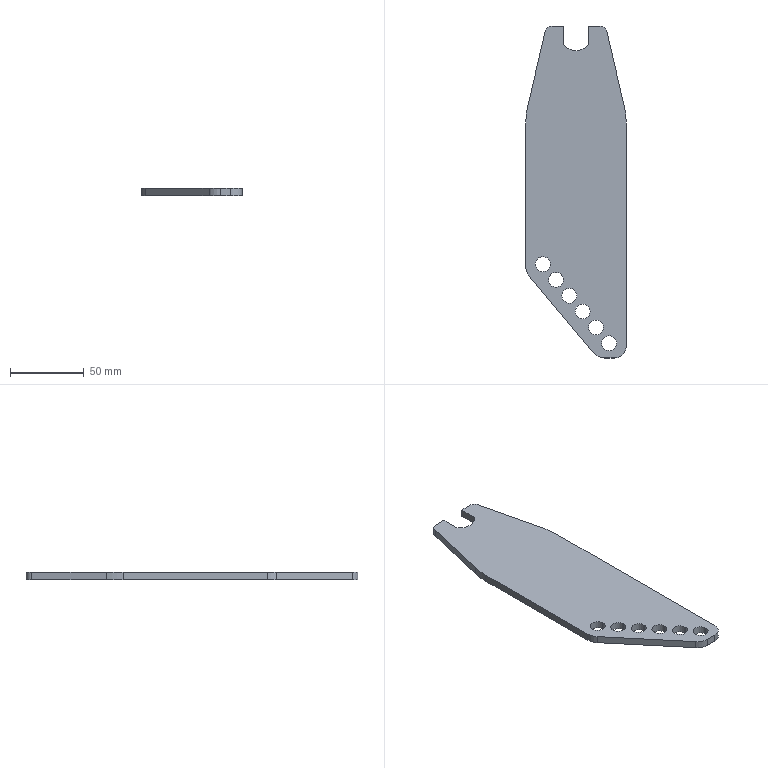Part | SolidWorks | features Fillet 5, ICE 4, Extrusion 1 | 1 solid | 32 faces | box 68 x 225 x 5 mm | volume 61427 mm3 | cylinder 20 | plane 12 | commonest cylinder face diameters 10.1 x12 10 x2 20 x2 100 x2 16 x1 21 x1
STEP:
#1=CARTESIAN_POINT('',(17.45,-102.5,0.));
#2=VERTEX_POINT('',#1);
#3=CARTESIAN_POINT('',(27.55,-102.5,0.));
#4=VERTEX_POINT('',#3);
#5=CARTESIAN_POINT('',(22.5,-102.5,0.));
#6=DIRECTION('',(0.,0.,1.));
#7=DIRECTION('',(1.,0.,0.));
#8=AXIS2_PLACEMENT_3D('',#5,#6,#7);
#9=CIRCLE('',#8,5.05);
#10=EDGE_CURVE('',#2,#4,#9,.T.);
#11=ORIENTED_EDGE('',*,*,#10,.F.);
#12=CARTESIAN_POINT('',(17.45,-102.5,5.));
#13=VERTEX_POINT('',#12);
#14=CARTESIAN_POINT('',(17.45,-102.5,-3.));
#15=DIRECTION('',(0.,0.,1.));
#16=VECTOR('',#15,1000.);
#17=LINE('',#14,#16);
#18=EDGE_CURVE('',#2,#13,#17,.T.);
#19=ORIENTED_EDGE('',*,*,#18,.T.);
#20=CARTESIAN_POINT('',(27.55,-102.5,5.));
#21=VERTEX_POINT('',#20);
#22=CARTESIAN_POINT('',(22.5,-102.5,5.));
#23=DIRECTION('',(0.,0.,1.));
#24=DIRECTION('',(1.,0.,0.));
#25=AXIS2_PLACEMENT_3D('',#22,#23,#24);
#26=CIRCLE('',#25,5.05);
#27=EDGE_CURVE('',#13,#21,#26,.T.);
#28=ORIENTED_EDGE('',*,*,#27,.T.);
#29=CARTESIAN_POINT('',(27.55,-102.5,-3.));
#30=DIRECTION('',(0.,0.,1.));
#31=VECTOR('',#30,1000.);
#32=LINE('',#29,#31);
#33=EDGE_CURVE('',#4,#21,#32,.T.);
#34=ORIENTED_EDGE('',*,*,#33,.F.);
#35=EDGE_LOOP('',(#11,#19,#28,#34));
#36=FACE_OUTER_BOUND('',#35,.T.);
#37=CARTESIAN_POINT('',(22.5,-102.5,-3.));
#38=DIRECTION('',(0.,0.,1.));
#39=DIRECTION('',(1.,0.,0.));
#40=AXIS2_PLACEMENT_3D('',#37,#38,#39);
#41=CYLINDRICAL_SURFACE('',#40,5.05);
#42=ADVANCED_FACE('',(#36),#41,.F.);
#43=CARTESIAN_POINT('',(8.451,-91.775,0.));
#44=VERTEX_POINT('',#43);
#45=CARTESIAN_POINT('',(18.551,-91.775,0.));
#46=VERTEX_POINT('',#45);
#47=CARTESIAN_POINT('',(13.501,-91.775,0.));
#48=DIRECTION('',(0.,0.,1.));
#49=DIRECTION('',(1.,0.,0.));
#50=AXIS2_PLACEMENT_3D('',#47,#48,#49);
#51=CIRCLE('',#50,5.05);
#52=EDGE_CURVE('',#44,#46,#51,.T.);
#53=ORIENTED_EDGE('',*,*,#52,.F.);
#54=CARTESIAN_POINT('',(8.451,-91.775,5.));
#55=VERTEX_POINT('',#54);
#56=CARTESIAN_POINT('',(8.451,-91.775,-3.));
#57=DIRECTION('',(0.,0.,1.));
#58=VECTOR('',#57,1000.);
#59=LINE('',#56,#58);
#60=EDGE_CURVE('',#44,#55,#59,.T.);
#61=ORIENTED_EDGE('',*,*,#60,.T.);
#62=CARTESIAN_POINT('',(18.551,-91.775,5.));
#63=VERTEX_POINT('',#62);
#64=CARTESIAN_POINT('',(13.501,-91.775,5.));
#65=DIRECTION('',(0.,0.,1.));
#66=DIRECTION('',(1.,0.,0.));
#67=AXIS2_PLACEMENT_3D('',#64,#65,#66);
#68=CIRCLE('',#67,5.05);
#69=EDGE_CURVE('',#55,#63,#68,.T.);
#70=ORIENTED_EDGE('',*,*,#69,.T.);
#71=CARTESIAN_POINT('',(18.551,-91.775,-3.));
#72=DIRECTION('',(0.,0.,1.));
#73=VECTOR('',#72,1000.);
#74=LINE('',#71,#73);
#75=EDGE_CURVE('',#46,#63,#74,.T.);
#76=ORIENTED_EDGE('',*,*,#75,.F.);
#77=EDGE_LOOP('',(#53,#61,#70,#76));
#78=FACE_OUTER_BOUND('',#77,.T.);
#79=CARTESIAN_POINT('',(13.501,-91.775,-3.));
#80=DIRECTION('',(0.,0.,1.));
#81=DIRECTION('',(1.,0.,0.));
#82=AXIS2_PLACEMENT_3D('',#79,#80,#81);
#83=CYLINDRICAL_SURFACE('',#82,5.05);
#84=ADVANCED_FACE('',(#78),#83,.F.);
#85=CARTESIAN_POINT('',(-0.5481,-81.051,0.));
#86=VERTEX_POINT('',#85);
#87=CARTESIAN_POINT('',(9.552,-81.051,0.));
#88=VERTEX_POINT('',#87);
#89=CARTESIAN_POINT('',(4.502,-81.051,0.));
#90=DIRECTION('',(0.,0.,1.));
#91=DIRECTION('',(1.,0.,0.));
#92=AXIS2_PLACEMENT_3D('',#89,#90,#91);
#93=CIRCLE('',#92,5.05);
#94=EDGE_CURVE('',#86,#88,#93,.T.);
#95=ORIENTED_EDGE('',*,*,#94,.F.);
#96=CARTESIAN_POINT('',(-0.5481,-81.051,5.));
#97=VERTEX_POINT('',#96);
#98=CARTESIAN_POINT('',(-0.5481,-81.051,-3.));
#99=DIRECTION('',(0.,0.,1.));
#100=VECTOR('',#99,1000.);
#101=LINE('',#98,#100);
#102=EDGE_CURVE('',#86,#97,#101,.T.);
#103=ORIENTED_EDGE('',*,*,#102,.T.);
#104=CARTESIAN_POINT('',(9.552,-81.051,5.));
#105=VERTEX_POINT('',#104);
#106=CARTESIAN_POINT('',(4.502,-81.051,5.));
#107=DIRECTION('',(0.,0.,1.));
#108=DIRECTION('',(1.,0.,0.));
#109=AXIS2_PLACEMENT_3D('',#106,#107,#108);
#110=CIRCLE('',#109,5.05);
#111=EDGE_CURVE('',#97,#105,#110,.T.);
#112=ORIENTED_EDGE('',*,*,#111,.T.);
#113=CARTESIAN_POINT('',(9.552,-81.051,-3.));
#114=DIRECTION('',(0.,0.,1.));
#115=VECTOR('',#114,1000.);
#116=LINE('',#113,#115);
#117=EDGE_CURVE('',#88,#105,#116,.T.);
#118=ORIENTED_EDGE('',*,*,#117,.F.);
#119=EDGE_LOOP('',(#95,#103,#112,#118));
#120=FACE_OUTER_BOUND('',#119,.T.);
#121=CARTESIAN_POINT('',(4.502,-81.051,-3.));
#122=DIRECTION('',(0.,0.,1.));
#123=DIRECTION('',(1.,0.,0.));
#124=AXIS2_PLACEMENT_3D('',#121,#122,#123);
#125=CYLINDRICAL_SURFACE('',#124,5.05);
#126=ADVANCED_FACE('',(#120),#125,.F.);
#127=CARTESIAN_POINT('',(-9.547,-70.326,0.));
#128=VERTEX_POINT('',#127);
#129=CARTESIAN_POINT('',(0.5529,-70.326,0.));
#130=VERTEX_POINT('',#129);
#131=CARTESIAN_POINT('',(-4.497,-70.326,0.));
#132=DIRECTION('',(0.,0.,1.));
#133=DIRECTION('',(1.,0.,0.));
#134=AXIS2_PLACEMENT_3D('',#131,#132,#133);
#135=CIRCLE('',#134,5.05);
#136=EDGE_CURVE('',#128,#130,#135,.T.);
#137=ORIENTED_EDGE('',*,*,#136,.F.);
#138=CARTESIAN_POINT('',(-9.547,-70.326,5.));
#139=VERTEX_POINT('',#138);
#140=CARTESIAN_POINT('',(-9.547,-70.326,-3.));
#141=DIRECTION('',(0.,0.,1.));
#142=VECTOR('',#141,1000.);
#143=LINE('',#140,#142);
#144=EDGE_CURVE('',#128,#139,#143,.T.);
#145=ORIENTED_EDGE('',*,*,#144,.T.);
#146=CARTESIAN_POINT('',(0.5529,-70.326,5.));
#147=VERTEX_POINT('',#146);
#148=CARTESIAN_POINT('',(-4.497,-70.326,5.));
#149=DIRECTION('',(0.,0.,1.));
#150=DIRECTION('',(1.,0.,0.));
#151=AXIS2_PLACEMENT_3D('',#148,#149,#150);
#152=CIRCLE('',#151,5.05);
#153=EDGE_CURVE('',#139,#147,#152,.T.);
#154=ORIENTED_EDGE('',*,*,#153,.T.);
#155=CARTESIAN_POINT('',(0.5529,-70.326,-3.));
#156=DIRECTION('',(0.,0.,1.));
#157=VECTOR('',#156,1000.);
#158=LINE('',#155,#157);
#159=EDGE_CURVE('',#130,#147,#158,.T.);
#160=ORIENTED_EDGE('',*,*,#159,.F.);
#161=EDGE_LOOP('',(#137,#145,#154,#160));
#162=FACE_OUTER_BOUND('',#161,.T.);
#163=CARTESIAN_POINT('',(-4.497,-70.326,-3.));
#164=DIRECTION('',(0.,0.,1.));
#165=DIRECTION('',(1.,0.,0.));
#166=AXIS2_PLACEMENT_3D('',#163,#164,#165);
#167=CYLINDRICAL_SURFACE('',#166,5.05);
#168=ADVANCED_FACE('',(#162),#167,.F.);
#169=CARTESIAN_POINT('',(-18.546,-59.602,0.));
#170=VERTEX_POINT('',#169);
#171=CARTESIAN_POINT('',(-8.446,-59.602,0.));
#172=VERTEX_POINT('',#171);
#173=CARTESIAN_POINT('',(-13.496,-59.602,0.));
#174=DIRECTION('',(0.,0.,1.));
#175=DIRECTION('',(1.,0.,0.));
#176=AXIS2_PLACEMENT_3D('',#173,#174,#175);
#177=CIRCLE('',#176,5.05);
#178=EDGE_CURVE('',#170,#172,#177,.T.);
#179=ORIENTED_EDGE('',*,*,#178,.F.);
#180=CARTESIAN_POINT('',(-18.546,-59.602,5.));
#181=VERTEX_POINT('',#180);
#182=CARTESIAN_POINT('',(-18.546,-59.602,-3.));
#183=DIRECTION('',(0.,0.,1.));
#184=VECTOR('',#183,1000.);
#185=LINE('',#182,#184);
#186=EDGE_CURVE('',#170,#181,#185,.T.);
#187=ORIENTED_EDGE('',*,*,#186,.T.);
#188=CARTESIAN_POINT('',(-8.446,-59.602,5.));
#189=VERTEX_POINT('',#188);
#190=CARTESIAN_POINT('',(-13.496,-59.602,5.));
#191=DIRECTION('',(0.,0.,1.));
#192=DIRECTION('',(1.,0.,0.));
#193=AXIS2_PLACEMENT_3D('',#190,#191,#192);
#194=CIRCLE('',#193,5.05);
#195=EDGE_CURVE('',#181,#189,#194,.T.);
#196=ORIENTED_EDGE('',*,*,#195,.T.);
#197=CARTESIAN_POINT('',(-8.446,-59.602,-3.));
#198=DIRECTION('',(0.,0.,1.));
#199=VECTOR('',#198,1000.);
#200=LINE('',#197,#199);
#201=EDGE_CURVE('',#172,#189,#200,.T.);
#202=ORIENTED_EDGE('',*,*,#201,.F.);
#203=EDGE_LOOP('',(#179,#187,#196,#202));
#204=FACE_OUTER_BOUND('',#203,.T.);
#205=CARTESIAN_POINT('',(-13.496,-59.602,-3.));
#206=DIRECTION('',(0.,0.,1.));
#207=DIRECTION('',(1.,0.,0.));
#208=AXIS2_PLACEMENT_3D('',#205,#206,#207);
#209=CYLINDRICAL_SURFACE('',#208,5.05);
#210=ADVANCED_FACE('',(#204),#209,.F.);
#211=CARTESIAN_POINT('',(-27.545,-48.877,0.));
#212=VERTEX_POINT('',#211);
#213=CARTESIAN_POINT('',(-17.445,-48.877,0.));
#214=VERTEX_POINT('',#213);
#215=CARTESIAN_POINT('',(-22.495,-48.877,0.));
#216=DIRECTION('',(0.,0.,1.));
#217=DIRECTION('',(1.,0.,0.));
#218=AXIS2_PLACEMENT_3D('',#215,#216,#217);
#219=CIRCLE('',#218,5.05);
#220=EDGE_CURVE('',#212,#214,#219,.T.);
#221=ORIENTED_EDGE('',*,*,#220,.F.);
#222=CARTESIAN_POINT('',(-27.545,-48.877,5.));
#223=VERTEX_POINT('',#222);
#224=CARTESIAN_POINT('',(-27.545,-48.877,-3.));
#225=DIRECTION('',(0.,0.,1.));
#226=VECTOR('',#225,1000.);
#227=LINE('',#224,#226);
#228=EDGE_CURVE('',#212,#223,#227,.T.);
#229=ORIENTED_EDGE('',*,*,#228,.T.);
#230=CARTESIAN_POINT('',(-17.445,-48.877,5.));
#231=VERTEX_POINT('',#230);
#232=CARTESIAN_POINT('',(-22.495,-48.877,5.));
#233=DIRECTION('',(0.,0.,1.));
#234=DIRECTION('',(1.,0.,0.));
#235=AXIS2_PLACEMENT_3D('',#232,#233,#234);
#236=CIRCLE('',#235,5.05);
#237=EDGE_CURVE('',#223,#231,#236,.T.);
#238=ORIENTED_EDGE('',*,*,#237,.T.);
#239=CARTESIAN_POINT('',(-17.445,-48.877,-3.));
#240=DIRECTION('',(0.,0.,1.));
#241=VECTOR('',#240,1000.);
#242=LINE('',#239,#241);
#243=EDGE_CURVE('',#214,#231,#242,.T.);
#244=ORIENTED_EDGE('',*,*,#243,.F.);
#245=EDGE_LOOP('',(#221,#229,#238,#244));
#246=FACE_OUTER_BOUND('',#245,.T.);
#247=CARTESIAN_POINT('',(-22.495,-48.877,-3.));
#248=DIRECTION('',(0.,0.,1.));
#249=DIRECTION('',(1.,0.,0.));
#250=AXIS2_PLACEMENT_3D('',#247,#248,#249);
#251=CYLINDRICAL_SURFACE('',#250,5.05);
#252=ADVANCED_FACE('',(#246),#251,.F.);
#253=CARTESIAN_POINT('',(16.032,112.5,5.));
#254=VERTEX_POINT('',#253);
#255=CARTESIAN_POINT('',(8.5,112.5,5.));
#256=VERTEX_POINT('',#255);
#257=CARTESIAN_POINT('',(-34.,112.5,5.));
#258=DIRECTION('',(-1.,0.,0.));
#259=VECTOR('',#258,1000.);
#260=LINE('',#257,#259);
#261=EDGE_CURVE('',#254,#256,#260,.T.);
#262=ORIENTED_EDGE('',*,*,#261,.F.);
#263=CARTESIAN_POINT('',(16.032,112.5,0.));
#264=VERTEX_POINT('',#263);
#265=CARTESIAN_POINT('',(16.032,112.5,5.));
#266=DIRECTION('',(0.,0.,-1.));
#267=VECTOR('',#266,1000.);
#268=LINE('',#265,#267);
#269=EDGE_CURVE('',#254,#264,#268,.T.);
#270=ORIENTED_EDGE('',*,*,#269,.T.);
#271=CARTESIAN_POINT('',(8.5,112.5,0.));
#272=VERTEX_POINT('',#271);
#273=CARTESIAN_POINT('',(-34.,112.5,0.));
#274=DIRECTION('',(-1.,0.,0.));
#275=VECTOR('',#274,1000.);
#276=LINE('',#273,#275);
#277=EDGE_CURVE('',#264,#272,#276,.T.);
#278=ORIENTED_EDGE('',*,*,#277,.T.);
#279=CARTESIAN_POINT('',(8.5,112.5,-3.));
#280=DIRECTION('',(0.,0.,1.));
#281=VECTOR('',#280,1000.);
#282=LINE('',#279,#281);
#283=EDGE_CURVE('',#272,#256,#282,.T.);
#284=ORIENTED_EDGE('',*,*,#283,.T.);
#285=EDGE_LOOP('',(#262,#270,#278,#284));
#286=FACE_OUTER_BOUND('',#285,.T.);
#287=CARTESIAN_POINT('',(-34.,112.5,5.));
#288=DIRECTION('',(0.,-1.,0.));
#289=DIRECTION('',(0.,0.,-1.));
#290=AXIS2_PLACEMENT_3D('',#287,#288,#289);
#291=PLANE('',#290);
#292=ADVANCED_FACE('',(#286),#291,.F.);
#293=CARTESIAN_POINT('',(34.,-104.5,0.));
#294=VERTEX_POINT('',#293);
#295=CARTESIAN_POINT('',(34.,46.744,0.));
#296=VERTEX_POINT('',#295);
#297=CARTESIAN_POINT('',(34.,112.5,0.));
#298=DIRECTION('',(0.,1.,0.));
#299=VECTOR('',#298,1000.);
#300=LINE('',#297,#299);
#301=EDGE_CURVE('',#294,#296,#300,.T.);
#302=ORIENTED_EDGE('',*,*,#301,.T.);
#303=CARTESIAN_POINT('',(34.,46.744,5.));
#304=VERTEX_POINT('',#303);
#305=CARTESIAN_POINT('',(34.,46.744,5.));
#306=DIRECTION('',(0.,0.,1.));
#307=VECTOR('',#306,1000.);
#308=LINE('',#305,#307);
#309=EDGE_CURVE('',#296,#304,#308,.T.);
#310=ORIENTED_EDGE('',*,*,#309,.T.);
#311=CARTESIAN_POINT('',(34.,-104.5,5.));
#312=VERTEX_POINT('',#311);
#313=CARTESIAN_POINT('',(34.,112.5,5.));
#314=DIRECTION('',(0.,1.,0.));
#315=VECTOR('',#314,1000.);
#316=LINE('',#313,#315);
#317=EDGE_CURVE('',#312,#304,#316,.T.);
#318=ORIENTED_EDGE('',*,*,#317,.F.);
#319=CARTESIAN_POINT('',(34.,-104.5,5.));
#320=DIRECTION('',(0.,0.,-1.));
#321=VECTOR('',#320,1000.);
#322=LINE('',#319,#321);
#323=EDGE_CURVE('',#312,#294,#322,.T.);
#324=ORIENTED_EDGE('',*,*,#323,.T.);
#325=EDGE_LOOP('',(#302,#310,#318,#324));
#326=FACE_OUTER_BOUND('',#325,.T.);
#327=CARTESIAN_POINT('',(34.,112.5,5.));
#328=DIRECTION('',(-1.,0.,0.));
#329=DIRECTION('',(0.,-1.,0.));
#330=AXIS2_PLACEMENT_3D('',#327,#328,#329);
#331=PLANE('',#330);
#332=ADVANCED_FACE('',(#326),#331,.F.);
#333=CARTESIAN_POINT('',(-8.5,112.5,0.));
#334=VERTEX_POINT('',#333);
#335=CARTESIAN_POINT('',(-16.032,112.5,0.));
#336=VERTEX_POINT('',#335);
#337=CARTESIAN_POINT('',(-34.,112.5,0.));
#338=DIRECTION('',(-1.,0.,0.));
#339=VECTOR('',#338,1000.);
#340=LINE('',#337,#339);
#341=EDGE_CURVE('',#334,#336,#340,.T.);
#342=ORIENTED_EDGE('',*,*,#341,.T.);
#343=CARTESIAN_POINT('',(-16.032,112.5,5.));
#344=VERTEX_POINT('',#343);
#345=CARTESIAN_POINT('',(-16.032,112.5,5.));
#346=DIRECTION('',(0.,0.,1.));
#347=VECTOR('',#346,1000.);
#348=LINE('',#345,#347);
#349=EDGE_CURVE('',#336,#344,#348,.T.);
#350=ORIENTED_EDGE('',*,*,#349,.T.);
#351=CARTESIAN_POINT('',(-8.5,112.5,5.));
#352=VERTEX_POINT('',#351);
#353=CARTESIAN_POINT('',(-34.,112.5,5.));
#354=DIRECTION('',(-1.,0.,0.));
#355=VECTOR('',#354,1000.);
#356=LINE('',#353,#355);
#357=EDGE_CURVE('',#352,#344,#356,.T.);
#358=ORIENTED_EDGE('',*,*,#357,.F.);
#359=CARTESIAN_POINT('',(-8.5,112.5,-3.));
#360=DIRECTION('',(0.,0.,1.));
#361=VECTOR('',#360,1000.);
#362=LINE('',#359,#361);
#363=EDGE_CURVE('',#334,#352,#362,.T.);
#364=ORIENTED_EDGE('',*,*,#363,.F.);
#365=EDGE_LOOP('',(#342,#350,#358,#364));
#366=FACE_OUTER_BOUND('',#365,.T.);
#367=CARTESIAN_POINT('',(-34.,112.5,5.));
#368=DIRECTION('',(0.,-1.,0.));
#369=DIRECTION('',(0.,0.,-1.));
#370=AXIS2_PLACEMENT_3D('',#367,#368,#369);
#371=PLANE('',#370);
#372=ADVANCED_FACE('',(#366),#371,.F.);
#373=CARTESIAN_POINT('',(-34.,46.744,5.));
#374=VERTEX_POINT('',#373);
#375=CARTESIAN_POINT('',(-34.,-50.973,5.));
#376=VERTEX_POINT('',#375);
#377=CARTESIAN_POINT('',(-34.,112.5,5.));
#378=DIRECTION('',(0.,-1.,0.));
#379=VECTOR('',#378,1000.);
#380=LINE('',#377,#379);
#381=EDGE_CURVE('',#374,#376,#380,.T.);
#382=ORIENTED_EDGE('',*,*,#381,.F.);
#383=CARTESIAN_POINT('',(-34.,46.744,0.));
#384=VERTEX_POINT('',#383);
#385=CARTESIAN_POINT('',(-34.,46.744,5.));
#386=DIRECTION('',(0.,0.,-1.));
#387=VECTOR('',#386,1000.);
#388=LINE('',#385,#387);
#389=EDGE_CURVE('',#374,#384,#388,.T.);
#390=ORIENTED_EDGE('',*,*,#389,.T.);
#391=CARTESIAN_POINT('',(-34.,-50.973,0.));
#392=VERTEX_POINT('',#391);
#393=CARTESIAN_POINT('',(-34.,112.5,0.));
#394=DIRECTION('',(0.,-1.,0.));
#395=VECTOR('',#394,1000.);
#396=LINE('',#393,#395);
#397=EDGE_CURVE('',#384,#392,#396,.T.);
#398=ORIENTED_EDGE('',*,*,#397,.T.);
#399=CARTESIAN_POINT('',(-34.,-50.973,5.));
#400=DIRECTION('',(0.,0.,1.));
#401=VECTOR('',#400,1000.);
#402=LINE('',#399,#401);
#403=EDGE_CURVE('',#392,#376,#402,.T.);
#404=ORIENTED_EDGE('',*,*,#403,.T.);
#405=EDGE_LOOP('',(#382,#390,#398,#404));
#406=FACE_OUTER_BOUND('',#405,.T.);
#407=CARTESIAN_POINT('',(-34.,112.5,5.));
#408=DIRECTION('',(1.,0.,0.));
#409=DIRECTION('',(0.,1.,0.));
#410=AXIS2_PLACEMENT_3D('',#407,#408,#409);
#411=PLANE('',#410);
#412=ADVANCED_FACE('',(#406),#411,.F.);
#413=CARTESIAN_POINT('',(19.236,-112.5,5.));
#414=VERTEX_POINT('',#413);
#415=CARTESIAN_POINT('',(26.,-112.5,5.));
#416=VERTEX_POINT('',#415);
#417=CARTESIAN_POINT('',(-34.,-112.5,5.));
#418=DIRECTION('',(1.,0.,0.));
#419=VECTOR('',#418,1000.);
#420=LINE('',#417,#419);
#421=EDGE_CURVE('',#414,#416,#420,.T.);
#422=ORIENTED_EDGE('',*,*,#421,.F.);
#423=CARTESIAN_POINT('',(19.236,-112.5,0.));
#424=VERTEX_POINT('',#423);
#425=CARTESIAN_POINT('',(19.236,-112.5,5.));
#426=DIRECTION('',(0.,0.,-1.));
#427=VECTOR('',#426,1000.);
#428=LINE('',#425,#427);
#429=EDGE_CURVE('',#414,#424,#428,.T.);
#430=ORIENTED_EDGE('',*,*,#429,.T.);
#431=CARTESIAN_POINT('',(26.,-112.5,0.));
#432=VERTEX_POINT('',#431);
#433=CARTESIAN_POINT('',(-34.,-112.5,0.));
#434=DIRECTION('',(1.,0.,0.));
#435=VECTOR('',#434,1000.);
#436=LINE('',#433,#435);
#437=EDGE_CURVE('',#424,#432,#436,.T.);
#438=ORIENTED_EDGE('',*,*,#437,.T.);
#439=CARTESIAN_POINT('',(26.,-112.5,5.));
#440=DIRECTION('',(0.,0.,1.));
#441=VECTOR('',#440,1000.);
#442=LINE('',#439,#441);
#443=EDGE_CURVE('',#432,#416,#442,.T.);
#444=ORIENTED_EDGE('',*,*,#443,.T.);
#445=EDGE_LOOP('',(#422,#430,#438,#444));
#446=FACE_OUTER_BOUND('',#445,.T.);
#447=CARTESIAN_POINT('',(-34.,-112.5,5.));
#448=DIRECTION('',(0.,1.,0.));
#449=DIRECTION('',(0.,0.,1.));
#450=AXIS2_PLACEMENT_3D('',#447,#448,#449);
#451=PLANE('',#450);
#452=ADVANCED_FACE('',(#446),#451,.F.);
#453=ORIENTED_EDGE('',*,*,#317,.T.);
#454=CARTESIAN_POINT('',(32.692,58.105,5.));
#455=VERTEX_POINT('',#454);
#456=CARTESIAN_POINT('',(-16.,46.744,5.));
#457=DIRECTION('',(0.,0.,1.));
#458=DIRECTION('',(1.,0.,0.));
#459=AXIS2_PLACEMENT_3D('',#456,#457,#458);
#460=CIRCLE('',#459,50.);
#461=EDGE_CURVE('',#304,#455,#460,.T.);
#462=ORIENTED_EDGE('',*,*,#461,.T.);
#463=CARTESIAN_POINT('',(20.902,108.636,5.));
#464=VERTEX_POINT('',#463);
#465=CARTESIAN_POINT('',(20.,112.5,5.));
#466=DIRECTION('',(0.2272,-0.9738,0.));
#467=VECTOR('',#466,1000.);
#468=LINE('',#465,#467);
#469=EDGE_CURVE('',#464,#455,#468,.T.);
#470=ORIENTED_EDGE('',*,*,#469,.F.);
#471=CARTESIAN_POINT('',(16.032,107.5,5.));
#472=DIRECTION('',(0.,0.,1.));
#473=DIRECTION('',(1.,0.,0.));
#474=AXIS2_PLACEMENT_3D('',#471,#472,#473);
#475=CIRCLE('',#474,5.);
#476=EDGE_CURVE('',#464,#254,#475,.T.);
#477=ORIENTED_EDGE('',*,*,#476,.T.);
#478=ORIENTED_EDGE('',*,*,#261,.T.);
#479=CARTESIAN_POINT('',(8.5,100.171,5.));
#480=VERTEX_POINT('',#479);
#481=CARTESIAN_POINT('',(8.5,112.5,5.));
#482=DIRECTION('',(0.,1.,0.));
#483=VECTOR('',#482,1000.);
#484=LINE('',#481,#483);
#485=EDGE_CURVE('',#480,#256,#484,.T.);
#486=ORIENTED_EDGE('',*,*,#485,.F.);
#487=CARTESIAN_POINT('',(-8.5,100.171,5.));
#488=VERTEX_POINT('',#487);
#489=CARTESIAN_POINT('',(0.,106.336,5.));
#490=DIRECTION('',(0.,0.,1.));
#491=DIRECTION('',(1.,0.,0.));
#492=AXIS2_PLACEMENT_3D('',#489,#490,#491);
#493=CIRCLE('',#492,10.5);
#494=EDGE_CURVE('',#488,#480,#493,.T.);
#495=ORIENTED_EDGE('',*,*,#494,.F.);
#496=CARTESIAN_POINT('',(-8.5,112.5,5.));
#497=DIRECTION('',(0.,-1.,0.));
#498=VECTOR('',#497,1000.);
#499=LINE('',#496,#498);
#500=EDGE_CURVE('',#352,#488,#499,.T.);
#501=ORIENTED_EDGE('',*,*,#500,.F.);
#502=ORIENTED_EDGE('',*,*,#357,.T.);
#503=CARTESIAN_POINT('',(-20.902,108.636,5.));
#504=VERTEX_POINT('',#503);
#505=CARTESIAN_POINT('',(-16.032,107.5,5.));
#506=DIRECTION('',(0.,0.,1.));
#507=DIRECTION('',(1.,0.,0.));
#508=AXIS2_PLACEMENT_3D('',#505,#506,#507);
#509=CIRCLE('',#508,5.);
#510=EDGE_CURVE('',#344,#504,#509,.T.);
#511=ORIENTED_EDGE('',*,*,#510,.T.);
#512=CARTESIAN_POINT('',(-32.692,58.105,5.));
#513=VERTEX_POINT('',#512);
#514=CARTESIAN_POINT('',(-20.,112.5,5.));
#515=DIRECTION('',(0.2272,0.9738,0.));
#516=VECTOR('',#515,1000.);
#517=LINE('',#514,#516);
#518=EDGE_CURVE('',#513,#504,#517,.T.);
#519=ORIENTED_EDGE('',*,*,#518,.F.);
#520=CARTESIAN_POINT('',(16.,46.744,5.));
#521=DIRECTION('',(0.,0.,1.));
#522=DIRECTION('',(1.,0.,0.));
#523=AXIS2_PLACEMENT_3D('',#520,#521,#522);
#524=CIRCLE('',#523,50.);
#525=EDGE_CURVE('',#513,#374,#524,.T.);
#526=ORIENTED_EDGE('',*,*,#525,.T.);
#527=ORIENTED_EDGE('',*,*,#381,.T.);
#528=CARTESIAN_POINT('',(-31.66,-57.401,5.));
#529=VERTEX_POINT('',#528);
#530=CARTESIAN_POINT('',(-24.,-50.973,5.));
#531=DIRECTION('',(0.,0.,1.));
#532=DIRECTION('',(1.,0.,0.));
#533=AXIS2_PLACEMENT_3D('',#530,#531,#532);
#534=CIRCLE('',#533,10.);
#535=EDGE_CURVE('',#376,#529,#534,.T.);
#536=ORIENTED_EDGE('',*,*,#535,.T.);
#537=CARTESIAN_POINT('',(11.576,-108.928,5.));
#538=VERTEX_POINT('',#537);
#539=CARTESIAN_POINT('',(14.573,-112.5,5.));
#540=DIRECTION('',(-0.6428,0.766,0.));
#541=VECTOR('',#540,1000.);
#542=LINE('',#539,#541);
#543=EDGE_CURVE('',#538,#529,#542,.T.);
#544=ORIENTED_EDGE('',*,*,#543,.F.);
#545=CARTESIAN_POINT('',(19.236,-102.5,5.));
#546=DIRECTION('',(0.,0.,1.));
#547=DIRECTION('',(1.,0.,0.));
#548=AXIS2_PLACEMENT_3D('',#545,#546,#547);
#549=CIRCLE('',#548,10.);
#550=EDGE_CURVE('',#538,#414,#549,.T.);
#551=ORIENTED_EDGE('',*,*,#550,.T.);
#552=ORIENTED_EDGE('',*,*,#421,.T.);
#553=CARTESIAN_POINT('',(26.,-104.5,5.));
#554=DIRECTION('',(0.,0.,1.));
#555=DIRECTION('',(1.,0.,0.));
#556=AXIS2_PLACEMENT_3D('',#553,#554,#555);
#557=CIRCLE('',#556,8.);
#558=EDGE_CURVE('',#416,#312,#557,.T.);
#559=ORIENTED_EDGE('',*,*,#558,.T.);
#560=EDGE_LOOP('',(#453,#462,#470,#477,#478,#486,#495,#501,#502,#511,#519,#526,#527,#536,#544,#551,#552,#559));
#561=FACE_OUTER_BOUND('',#560,.T.);
#562=CARTESIAN_POINT('',(22.5,-102.5,5.));
#563=DIRECTION('',(0.,0.,1.));
#564=DIRECTION('',(1.,0.,0.));
#565=AXIS2_PLACEMENT_3D('',#562,#563,#564);
#566=CIRCLE('',#565,5.05);
#567=EDGE_CURVE('',#21,#13,#566,.T.);
#568=ORIENTED_EDGE('',*,*,#567,.F.);
#569=ORIENTED_EDGE('',*,*,#27,.F.);
#570=EDGE_LOOP('',(#568,#569));
#571=FACE_BOUND('',#570,.T.);
#572=CARTESIAN_POINT('',(13.501,-91.775,5.));
#573=DIRECTION('',(0.,0.,1.));
#574=DIRECTION('',(1.,0.,0.));
#575=AXIS2_PLACEMENT_3D('',#572,#573,#574);
#576=CIRCLE('',#575,5.05);
#577=EDGE_CURVE('',#63,#55,#576,.T.);
#578=ORIENTED_EDGE('',*,*,#577,.F.);
#579=ORIENTED_EDGE('',*,*,#69,.F.);
#580=EDGE_LOOP('',(#578,#579));
#581=FACE_BOUND('',#580,.T.);
#582=CARTESIAN_POINT('',(4.502,-81.051,5.));
#583=DIRECTION('',(0.,0.,1.));
#584=DIRECTION('',(1.,0.,0.));
#585=AXIS2_PLACEMENT_3D('',#582,#583,#584);
#586=CIRCLE('',#585,5.05);
#587=EDGE_CURVE('',#105,#97,#586,.T.);
#588=ORIENTED_EDGE('',*,*,#587,.F.);
#589=ORIENTED_EDGE('',*,*,#111,.F.);
#590=EDGE_LOOP('',(#588,#589));
#591=FACE_BOUND('',#590,.T.);
#592=CARTESIAN_POINT('',(-4.497,-70.326,5.));
#593=DIRECTION('',(0.,0.,1.));
#594=DIRECTION('',(1.,0.,0.));
#595=AXIS2_PLACEMENT_3D('',#592,#593,#594);
#596=CIRCLE('',#595,5.05);
#597=EDGE_CURVE('',#147,#139,#596,.T.);
#598=ORIENTED_EDGE('',*,*,#597,.F.);
#599=ORIENTED_EDGE('',*,*,#153,.F.);
#600=EDGE_LOOP('',(#598,#599));
#601=FACE_BOUND('',#600,.T.);
#602=CARTESIAN_POINT('',(-13.496,-59.602,5.));
#603=DIRECTION('',(0.,0.,1.));
#604=DIRECTION('',(1.,0.,0.));
#605=AXIS2_PLACEMENT_3D('',#602,#603,#604);
#606=CIRCLE('',#605,5.05);
#607=EDGE_CURVE('',#189,#181,#606,.T.);
#608=ORIENTED_EDGE('',*,*,#607,.F.);
#609=ORIENTED_EDGE('',*,*,#195,.F.);
#610=EDGE_LOOP('',(#608,#609));
#611=FACE_BOUND('',#610,.T.);
#612=CARTESIAN_POINT('',(-22.495,-48.877,5.));
#613=DIRECTION('',(0.,0.,1.));
#614=DIRECTION('',(1.,0.,0.));
#615=AXIS2_PLACEMENT_3D('',#612,#613,#614);
#616=CIRCLE('',#615,5.05);
#617=EDGE_CURVE('',#231,#223,#616,.T.);
#618=ORIENTED_EDGE('',*,*,#617,.F.);
#619=ORIENTED_EDGE('',*,*,#237,.F.);
#620=EDGE_LOOP('',(#618,#619));
#621=FACE_BOUND('',#620,.T.);
#622=CARTESIAN_POINT('',(0.,0.,5.));
#623=DIRECTION('',(0.,0.,1.));
#624=DIRECTION('',(1.,0.,0.));
#625=AXIS2_PLACEMENT_3D('',#622,#623,#624);
#626=PLANE('',#625);
#627=ADVANCED_FACE('',(#561,#571,#581,#591,#601,#611,#621),#626,.T.);
#628=CARTESIAN_POINT('',(22.5,-102.5,0.));
#629=DIRECTION('',(0.,0.,1.));
#630=DIRECTION('',(1.,0.,0.));
#631=AXIS2_PLACEMENT_3D('',#628,#629,#630);
#632=CIRCLE('',#631,5.05);
#633=EDGE_CURVE('',#4,#2,#632,.T.);
#634=ORIENTED_EDGE('',*,*,#633,.T.);
#635=ORIENTED_EDGE('',*,*,#10,.T.);
#636=EDGE_LOOP('',(#634,#635));
#637=FACE_BOUND('',#636,.T.);
#638=CARTESIAN_POINT('',(13.501,-91.775,0.));
#639=DIRECTION('',(0.,0.,1.));
#640=DIRECTION('',(1.,0.,0.));
#641=AXIS2_PLACEMENT_3D('',#638,#639,#640);
#642=CIRCLE('',#641,5.05);
#643=EDGE_CURVE('',#46,#44,#642,.T.);
#644=ORIENTED_EDGE('',*,*,#643,.T.);
#645=ORIENTED_EDGE('',*,*,#52,.T.);
#646=EDGE_LOOP('',(#644,#645));
#647=FACE_BOUND('',#646,.T.);
#648=CARTESIAN_POINT('',(4.502,-81.051,0.));
#649=DIRECTION('',(0.,0.,1.));
#650=DIRECTION('',(1.,0.,0.));
#651=AXIS2_PLACEMENT_3D('',#648,#649,#650);
#652=CIRCLE('',#651,5.05);
#653=EDGE_CURVE('',#88,#86,#652,.T.);
#654=ORIENTED_EDGE('',*,*,#653,.T.);
#655=ORIENTED_EDGE('',*,*,#94,.T.);
#656=EDGE_LOOP('',(#654,#655));
#657=FACE_BOUND('',#656,.T.);
#658=CARTESIAN_POINT('',(-4.497,-70.326,0.));
#659=DIRECTION('',(0.,0.,1.));
#660=DIRECTION('',(1.,0.,0.));
#661=AXIS2_PLACEMENT_3D('',#658,#659,#660);
#662=CIRCLE('',#661,5.05);
#663=EDGE_CURVE('',#130,#128,#662,.T.);
#664=ORIENTED_EDGE('',*,*,#663,.T.);
#665=ORIENTED_EDGE('',*,*,#136,.T.);
#666=EDGE_LOOP('',(#664,#665));
#667=FACE_BOUND('',#666,.T.);
#668=CARTESIAN_POINT('',(-13.496,-59.602,0.));
#669=DIRECTION('',(0.,0.,1.));
#670=DIRECTION('',(1.,0.,0.));
#671=AXIS2_PLACEMENT_3D('',#668,#669,#670);
#672=CIRCLE('',#671,5.05);
#673=EDGE_CURVE('',#172,#170,#672,.T.);
#674=ORIENTED_EDGE('',*,*,#673,.T.);
#675=ORIENTED_EDGE('',*,*,#178,.T.);
#676=EDGE_LOOP('',(#674,#675));
#677=FACE_BOUND('',#676,.T.);
#678=CARTESIAN_POINT('',(-22.495,-48.877,0.));
#679=DIRECTION('',(0.,0.,1.));
#680=DIRECTION('',(1.,0.,0.));
#681=AXIS2_PLACEMENT_3D('',#678,#679,#680);
#682=CIRCLE('',#681,5.05);
#683=EDGE_CURVE('',#214,#212,#682,.T.);
#684=ORIENTED_EDGE('',*,*,#683,.T.);
#685=ORIENTED_EDGE('',*,*,#220,.T.);
#686=EDGE_LOOP('',(#684,#685));
#687=FACE_BOUND('',#686,.T.);
#688=CARTESIAN_POINT('',(20.902,108.636,0.));
#689=VERTEX_POINT('',#688);
#690=CARTESIAN_POINT('',(32.692,58.105,0.));
#691=VERTEX_POINT('',#690);
#692=CARTESIAN_POINT('',(20.,112.5,0.));
#693=DIRECTION('',(0.2272,-0.9738,0.));
#694=VECTOR('',#693,1000.);
#695=LINE('',#692,#694);
#696=EDGE_CURVE('',#689,#691,#695,.T.);
#697=ORIENTED_EDGE('',*,*,#696,.T.);
#698=CARTESIAN_POINT('',(-16.,46.744,0.));
#699=DIRECTION('',(0.,0.,-1.));
#700=DIRECTION('',(1.,0.,0.));
#701=AXIS2_PLACEMENT_3D('',#698,#699,#700);
#702=CIRCLE('',#701,50.);
#703=EDGE_CURVE('',#691,#296,#702,.T.);
#704=ORIENTED_EDGE('',*,*,#703,.T.);
#705=ORIENTED_EDGE('',*,*,#301,.F.);
#706=CARTESIAN_POINT('',(26.,-104.5,0.));
#707=DIRECTION('',(0.,0.,-1.));
#708=DIRECTION('',(1.,0.,0.));
#709=AXIS2_PLACEMENT_3D('',#706,#707,#708);
#710=CIRCLE('',#709,8.);
#711=EDGE_CURVE('',#294,#432,#710,.T.);
#712=ORIENTED_EDGE('',*,*,#711,.T.);
#713=ORIENTED_EDGE('',*,*,#437,.F.);
#714=CARTESIAN_POINT('',(11.576,-108.928,0.));
#715=VERTEX_POINT('',#714);
#716=CARTESIAN_POINT('',(19.236,-102.5,0.));
#717=DIRECTION('',(0.,0.,-1.));
#718=DIRECTION('',(1.,0.,0.));
#719=AXIS2_PLACEMENT_3D('',#716,#717,#718);
#720=CIRCLE('',#719,10.);
#721=EDGE_CURVE('',#424,#715,#720,.T.);
#722=ORIENTED_EDGE('',*,*,#721,.T.);
#723=CARTESIAN_POINT('',(-31.66,-57.401,0.));
#724=VERTEX_POINT('',#723);
#725=CARTESIAN_POINT('',(14.573,-112.5,0.));
#726=DIRECTION('',(-0.6428,0.766,0.));
#727=VECTOR('',#726,1000.);
#728=LINE('',#725,#727);
#729=EDGE_CURVE('',#715,#724,#728,.T.);
#730=ORIENTED_EDGE('',*,*,#729,.T.);
#731=CARTESIAN_POINT('',(-24.,-50.973,0.));
#732=DIRECTION('',(0.,0.,-1.));
#733=DIRECTION('',(1.,0.,0.));
#734=AXIS2_PLACEMENT_3D('',#731,#732,#733);
#735=CIRCLE('',#734,10.);
#736=EDGE_CURVE('',#724,#392,#735,.T.);
#737=ORIENTED_EDGE('',*,*,#736,.T.);
#738=ORIENTED_EDGE('',*,*,#397,.F.);
#739=CARTESIAN_POINT('',(-32.692,58.105,0.));
#740=VERTEX_POINT('',#739);
#741=CARTESIAN_POINT('',(16.,46.744,0.));
#742=DIRECTION('',(0.,0.,-1.));
#743=DIRECTION('',(1.,0.,0.));
#744=AXIS2_PLACEMENT_3D('',#741,#742,#743);
#745=CIRCLE('',#744,50.);
#746=EDGE_CURVE('',#384,#740,#745,.T.);
#747=ORIENTED_EDGE('',*,*,#746,.T.);
#748=CARTESIAN_POINT('',(-20.902,108.636,0.));
#749=VERTEX_POINT('',#748);
#750=CARTESIAN_POINT('',(-20.,112.5,0.));
#751=DIRECTION('',(0.2272,0.9738,0.));
#752=VECTOR('',#751,1000.);
#753=LINE('',#750,#752);
#754=EDGE_CURVE('',#740,#749,#753,.T.);
#755=ORIENTED_EDGE('',*,*,#754,.T.);
#756=CARTESIAN_POINT('',(-16.032,107.5,0.));
#757=DIRECTION('',(0.,0.,-1.));
#758=DIRECTION('',(1.,0.,0.));
#759=AXIS2_PLACEMENT_3D('',#756,#757,#758);
#760=CIRCLE('',#759,5.);
#761=EDGE_CURVE('',#749,#336,#760,.T.);
#762=ORIENTED_EDGE('',*,*,#761,.T.);
#763=ORIENTED_EDGE('',*,*,#341,.F.);
#764=CARTESIAN_POINT('',(-8.5,100.171,0.));
#765=VERTEX_POINT('',#764);
#766=CARTESIAN_POINT('',(-8.5,0.,0.));
#767=DIRECTION('',(0.,-1.,0.));
#768=VECTOR('',#767,1000.);
#769=LINE('',#766,#768);
#770=EDGE_CURVE('',#334,#765,#769,.T.);
#771=ORIENTED_EDGE('',*,*,#770,.T.);
#772=CARTESIAN_POINT('',(8.5,100.171,0.));
#773=VERTEX_POINT('',#772);
#774=CARTESIAN_POINT('',(0.,106.336,0.));
#775=DIRECTION('',(0.,0.,1.));
#776=DIRECTION('',(1.,0.,0.));
#777=AXIS2_PLACEMENT_3D('',#774,#775,#776);
#778=CIRCLE('',#777,10.5);
#779=EDGE_CURVE('',#765,#773,#778,.T.);
#780=ORIENTED_EDGE('',*,*,#779,.T.);
#781=CARTESIAN_POINT('',(8.5,0.,0.));
#782=DIRECTION('',(0.,1.,0.));
#783=VECTOR('',#782,1000.);
#784=LINE('',#781,#783);
#785=EDGE_CURVE('',#773,#272,#784,.T.);
#786=ORIENTED_EDGE('',*,*,#785,.T.);
#787=ORIENTED_EDGE('',*,*,#277,.F.);
#788=CARTESIAN_POINT('',(16.032,107.5,0.));
#789=DIRECTION('',(0.,0.,-1.));
#790=DIRECTION('',(1.,0.,0.));
#791=AXIS2_PLACEMENT_3D('',#788,#789,#790);
#792=CIRCLE('',#791,5.);
#793=EDGE_CURVE('',#264,#689,#792,.T.);
#794=ORIENTED_EDGE('',*,*,#793,.T.);
#795=EDGE_LOOP('',(#697,#704,#705,#712,#713,#722,#730,#737,#738,#747,#755,#762,#763,#771,#780,#786,#787,#794));
#796=FACE_OUTER_BOUND('',#795,.T.);
#797=CARTESIAN_POINT('',(0.,0.,0.));
#798=DIRECTION('',(0.,0.,1.));
#799=DIRECTION('',(1.,0.,0.));
#800=AXIS2_PLACEMENT_3D('',#797,#798,#799);
#801=PLANE('',#800);
#802=ADVANCED_FACE('',(#637,#647,#657,#667,#677,#687,#796),#801,.F.);
#803=ORIENTED_EDGE('',*,*,#228,.F.);
#804=ORIENTED_EDGE('',*,*,#683,.F.);
#805=ORIENTED_EDGE('',*,*,#243,.T.);
#806=ORIENTED_EDGE('',*,*,#617,.T.);
#807=EDGE_LOOP('',(#803,#804,#805,#806));
#808=FACE_OUTER_BOUND('',#807,.T.);
#809=CARTESIAN_POINT('',(-22.495,-48.877,-3.));
#810=DIRECTION('',(0.,0.,1.));
#811=DIRECTION('',(1.,0.,0.));
#812=AXIS2_PLACEMENT_3D('',#809,#810,#811);
#813=CYLINDRICAL_SURFACE('',#812,5.05);
#814=ADVANCED_FACE('',(#808),#813,.F.);
#815=ORIENTED_EDGE('',*,*,#186,.F.);
#816=ORIENTED_EDGE('',*,*,#673,.F.);
#817=ORIENTED_EDGE('',*,*,#201,.T.);
#818=ORIENTED_EDGE('',*,*,#607,.T.);
#819=EDGE_LOOP('',(#815,#816,#817,#818));
#820=FACE_OUTER_BOUND('',#819,.T.);
#821=CARTESIAN_POINT('',(-13.496,-59.602,-3.));
#822=DIRECTION('',(0.,0.,1.));
#823=DIRECTION('',(1.,0.,0.));
#824=AXIS2_PLACEMENT_3D('',#821,#822,#823);
#825=CYLINDRICAL_SURFACE('',#824,5.05);
#826=ADVANCED_FACE('',(#820),#825,.F.);
#827=ORIENTED_EDGE('',*,*,#144,.F.);
#828=ORIENTED_EDGE('',*,*,#663,.F.);
#829=ORIENTED_EDGE('',*,*,#159,.T.);
#830=ORIENTED_EDGE('',*,*,#597,.T.);
#831=EDGE_LOOP('',(#827,#828,#829,#830));
#832=FACE_OUTER_BOUND('',#831,.T.);
#833=CARTESIAN_POINT('',(-4.497,-70.326,-3.));
#834=DIRECTION('',(0.,0.,1.));
#835=DIRECTION('',(1.,0.,0.));
#836=AXIS2_PLACEMENT_3D('',#833,#834,#835);
#837=CYLINDRICAL_SURFACE('',#836,5.05);
#838=ADVANCED_FACE('',(#832),#837,.F.);
#839=ORIENTED_EDGE('',*,*,#102,.F.);
#840=ORIENTED_EDGE('',*,*,#653,.F.);
#841=ORIENTED_EDGE('',*,*,#117,.T.);
#842=ORIENTED_EDGE('',*,*,#587,.T.);
#843=EDGE_LOOP('',(#839,#840,#841,#842));
#844=FACE_OUTER_BOUND('',#843,.T.);
#845=CARTESIAN_POINT('',(4.502,-81.051,-3.));
#846=DIRECTION('',(0.,0.,1.));
#847=DIRECTION('',(1.,0.,0.));
#848=AXIS2_PLACEMENT_3D('',#845,#846,#847);
#849=CYLINDRICAL_SURFACE('',#848,5.05);
#850=ADVANCED_FACE('',(#844),#849,.F.);
#851=ORIENTED_EDGE('',*,*,#60,.F.);
#852=ORIENTED_EDGE('',*,*,#643,.F.);
#853=ORIENTED_EDGE('',*,*,#75,.T.);
#854=ORIENTED_EDGE('',*,*,#577,.T.);
#855=EDGE_LOOP('',(#851,#852,#853,#854));
#856=FACE_OUTER_BOUND('',#855,.T.);
#857=CARTESIAN_POINT('',(13.501,-91.775,-3.));
#858=DIRECTION('',(0.,0.,1.));
#859=DIRECTION('',(1.,0.,0.));
#860=AXIS2_PLACEMENT_3D('',#857,#858,#859);
#861=CYLINDRICAL_SURFACE('',#860,5.05);
#862=ADVANCED_FACE('',(#856),#861,.F.);
#863=ORIENTED_EDGE('',*,*,#18,.F.);
#864=ORIENTED_EDGE('',*,*,#633,.F.);
#865=ORIENTED_EDGE('',*,*,#33,.T.);
#866=ORIENTED_EDGE('',*,*,#567,.T.);
#867=EDGE_LOOP('',(#863,#864,#865,#866));
#868=FACE_OUTER_BOUND('',#867,.T.);
#869=CARTESIAN_POINT('',(22.5,-102.5,-3.));
#870=DIRECTION('',(0.,0.,1.));
#871=DIRECTION('',(1.,0.,0.));
#872=AXIS2_PLACEMENT_3D('',#869,#870,#871);
#873=CYLINDRICAL_SURFACE('',#872,5.05);
#874=ADVANCED_FACE('',(#868),#873,.F.);
#875=ORIENTED_EDGE('',*,*,#558,.F.);
#876=ORIENTED_EDGE('',*,*,#443,.F.);
#877=ORIENTED_EDGE('',*,*,#711,.F.);
#878=ORIENTED_EDGE('',*,*,#323,.F.);
#879=EDGE_LOOP('',(#875,#876,#877,#878));
#880=FACE_OUTER_BOUND('',#879,.T.);
#881=CARTESIAN_POINT('',(26.,-104.5,5.));
#882=DIRECTION('',(0.,0.,-1.));
#883=DIRECTION('',(-1.,0.,0.));
#884=AXIS2_PLACEMENT_3D('',#881,#882,#883);
#885=CYLINDRICAL_SURFACE('',#884,8.);
#886=ADVANCED_FACE('',(#880),#885,.T.);
#887=ORIENTED_EDGE('',*,*,#543,.T.);
#888=CARTESIAN_POINT('',(-31.66,-57.401,0.));
#889=DIRECTION('',(0.,0.,-1.));
#890=VECTOR('',#889,1000.);
#891=LINE('',#888,#890);
#892=EDGE_CURVE('',#529,#724,#891,.T.);
#893=ORIENTED_EDGE('',*,*,#892,.T.);
#894=ORIENTED_EDGE('',*,*,#729,.F.);
#895=CARTESIAN_POINT('',(11.576,-108.928,0.));
#896=DIRECTION('',(0.,0.,1.));
#897=VECTOR('',#896,1000.);
#898=LINE('',#895,#897);
#899=EDGE_CURVE('',#715,#538,#898,.T.);
#900=ORIENTED_EDGE('',*,*,#899,.T.);
#901=EDGE_LOOP('',(#887,#893,#894,#900));
#902=FACE_OUTER_BOUND('',#901,.T.);
#903=CARTESIAN_POINT('',(14.573,-112.5,0.));
#904=DIRECTION('',(0.766,0.6428,0.));
#905=DIRECTION('',(-0.6428,0.766,0.));
#906=AXIS2_PLACEMENT_3D('',#903,#904,#905);
#907=PLANE('',#906);
#908=ADVANCED_FACE('',(#902),#907,.F.);
#909=ORIENTED_EDGE('',*,*,#721,.F.);
#910=ORIENTED_EDGE('',*,*,#429,.F.);
#911=ORIENTED_EDGE('',*,*,#550,.F.);
#912=ORIENTED_EDGE('',*,*,#899,.F.);
#913=EDGE_LOOP('',(#909,#910,#911,#912));
#914=FACE_OUTER_BOUND('',#913,.T.);
#915=CARTESIAN_POINT('',(19.236,-102.5,0.));
#916=DIRECTION('',(0.,0.,1.));
#917=DIRECTION('',(1.,0.,0.));
#918=AXIS2_PLACEMENT_3D('',#915,#916,#917);
#919=CYLINDRICAL_SURFACE('',#918,10.);
#920=ADVANCED_FACE('',(#914),#919,.T.);
#921=CARTESIAN_POINT('',(8.5,100.171,-3.));
#922=DIRECTION('',(0.,0.,1.));
#923=VECTOR('',#922,1000.);
#924=LINE('',#921,#923);
#925=EDGE_CURVE('',#773,#480,#924,.T.);
#926=ORIENTED_EDGE('',*,*,#925,.T.);
#927=ORIENTED_EDGE('',*,*,#485,.T.);
#928=ORIENTED_EDGE('',*,*,#283,.F.);
#929=ORIENTED_EDGE('',*,*,#785,.F.);
#930=EDGE_LOOP('',(#926,#927,#928,#929));
#931=FACE_OUTER_BOUND('',#930,.T.);
#932=CARTESIAN_POINT('',(8.5,112.5,-3.));
#933=DIRECTION('',(1.,0.,0.));
#934=DIRECTION('',(0.,1.,0.));
#935=AXIS2_PLACEMENT_3D('',#932,#933,#934);
#936=PLANE('',#935);
#937=ADVANCED_FACE('',(#931),#936,.F.);
#938=CARTESIAN_POINT('',(-8.5,100.171,-3.));
#939=DIRECTION('',(0.,0.,1.));
#940=VECTOR('',#939,1000.);
#941=LINE('',#938,#940);
#942=EDGE_CURVE('',#765,#488,#941,.T.);
#943=ORIENTED_EDGE('',*,*,#942,.T.);
#944=ORIENTED_EDGE('',*,*,#494,.T.);
#945=ORIENTED_EDGE('',*,*,#925,.F.);
#946=ORIENTED_EDGE('',*,*,#779,.F.);
#947=EDGE_LOOP('',(#943,#944,#945,#946));
#948=FACE_OUTER_BOUND('',#947,.T.);
#949=CARTESIAN_POINT('',(0.,106.336,-3.));
#950=DIRECTION('',(0.,0.,1.));
#951=DIRECTION('',(1.,0.,0.));
#952=AXIS2_PLACEMENT_3D('',#949,#950,#951);
#953=CYLINDRICAL_SURFACE('',#952,10.5);
#954=ADVANCED_FACE('',(#948),#953,.F.);
#955=ORIENTED_EDGE('',*,*,#363,.T.);
#956=ORIENTED_EDGE('',*,*,#500,.T.);
#957=ORIENTED_EDGE('',*,*,#942,.F.);
#958=ORIENTED_EDGE('',*,*,#770,.F.);
#959=EDGE_LOOP('',(#955,#956,#957,#958));
#960=FACE_OUTER_BOUND('',#959,.T.);
#961=CARTESIAN_POINT('',(-8.5,112.5,-3.));
#962=DIRECTION('',(-1.,0.,0.));
#963=DIRECTION('',(0.,-1.,0.));
#964=AXIS2_PLACEMENT_3D('',#961,#962,#963);
#965=PLANE('',#964);
#966=ADVANCED_FACE('',(#960),#965,.F.);
#967=ORIENTED_EDGE('',*,*,#736,.F.);
#968=ORIENTED_EDGE('',*,*,#892,.F.);
#969=ORIENTED_EDGE('',*,*,#535,.F.);
#970=ORIENTED_EDGE('',*,*,#403,.F.);
#971=EDGE_LOOP('',(#967,#968,#969,#970));
#972=FACE_OUTER_BOUND('',#971,.T.);
#973=CARTESIAN_POINT('',(-24.,-50.973,5.));
#974=DIRECTION('',(0.,0.,1.));
#975=DIRECTION('',(1.,0.,0.));
#976=AXIS2_PLACEMENT_3D('',#973,#974,#975);
#977=CYLINDRICAL_SURFACE('',#976,10.);
#978=ADVANCED_FACE('',(#972),#977,.T.);
#979=ORIENTED_EDGE('',*,*,#469,.T.);
#980=CARTESIAN_POINT('',(32.692,58.105,0.));
#981=DIRECTION('',(0.,0.,-1.));
#982=VECTOR('',#981,1000.);
#983=LINE('',#980,#982);
#984=EDGE_CURVE('',#455,#691,#983,.T.);
#985=ORIENTED_EDGE('',*,*,#984,.T.);
#986=ORIENTED_EDGE('',*,*,#696,.F.);
#987=CARTESIAN_POINT('',(20.902,108.636,0.));
#988=DIRECTION('',(0.,0.,1.));
#989=VECTOR('',#988,1000.);
#990=LINE('',#987,#989);
#991=EDGE_CURVE('',#689,#464,#990,.T.);
#992=ORIENTED_EDGE('',*,*,#991,.T.);
#993=EDGE_LOOP('',(#979,#985,#986,#992));
#994=FACE_OUTER_BOUND('',#993,.T.);
#995=CARTESIAN_POINT('',(20.,112.5,0.));
#996=DIRECTION('',(-0.9738,-0.2272,0.));
#997=DIRECTION('',(0.2272,-0.9738,0.));
#998=AXIS2_PLACEMENT_3D('',#995,#996,#997);
#999=PLANE('',#998);
#1000=ADVANCED_FACE('',(#994),#999,.F.);
#1001=ORIENTED_EDGE('',*,*,#754,.F.);
#1002=CARTESIAN_POINT('',(-32.692,58.105,0.));
#1003=DIRECTION('',(0.,0.,1.));
#1004=VECTOR('',#1003,1000.);
#1005=LINE('',#1002,#1004);
#1006=EDGE_CURVE('',#740,#513,#1005,.T.);
#1007=ORIENTED_EDGE('',*,*,#1006,.T.);
#1008=ORIENTED_EDGE('',*,*,#518,.T.);
#1009=CARTESIAN_POINT('',(-20.902,108.636,0.));
#1010=DIRECTION('',(0.,0.,-1.));
#1011=VECTOR('',#1010,1000.);
#1012=LINE('',#1009,#1011);
#1013=EDGE_CURVE('',#504,#749,#1012,.T.);
#1014=ORIENTED_EDGE('',*,*,#1013,.T.);
#1015=EDGE_LOOP('',(#1001,#1007,#1008,#1014));
#1016=FACE_OUTER_BOUND('',#1015,.T.);
#1017=CARTESIAN_POINT('',(-20.,112.5,0.));
#1018=DIRECTION('',(0.9738,-0.2272,0.));
#1019=DIRECTION('',(0.2272,0.9738,0.));
#1020=AXIS2_PLACEMENT_3D('',#1017,#1018,#1019);
#1021=PLANE('',#1020);
#1022=ADVANCED_FACE('',(#1016),#1021,.F.);
#1023=ORIENTED_EDGE('',*,*,#793,.F.);
#1024=ORIENTED_EDGE('',*,*,#269,.F.);
#1025=ORIENTED_EDGE('',*,*,#476,.F.);
#1026=ORIENTED_EDGE('',*,*,#991,.F.);
#1027=EDGE_LOOP('',(#1023,#1024,#1025,#1026));
#1028=FACE_OUTER_BOUND('',#1027,.T.);
#1029=CARTESIAN_POINT('',(16.032,107.5,0.));
#1030=DIRECTION('',(0.,0.,1.));
#1031=DIRECTION('',(1.,0.,0.));
#1032=AXIS2_PLACEMENT_3D('',#1029,#1030,#1031);
#1033=CYLINDRICAL_SURFACE('',#1032,5.);
#1034=ADVANCED_FACE('',(#1028),#1033,.T.);
#1035=ORIENTED_EDGE('',*,*,#761,.F.);
#1036=ORIENTED_EDGE('',*,*,#1013,.F.);
#1037=ORIENTED_EDGE('',*,*,#510,.F.);
#1038=ORIENTED_EDGE('',*,*,#349,.F.);
#1039=EDGE_LOOP('',(#1035,#1036,#1037,#1038));
#1040=FACE_OUTER_BOUND('',#1039,.T.);
#1041=CARTESIAN_POINT('',(-16.032,107.5,5.));
#1042=DIRECTION('',(0.,0.,1.));
#1043=DIRECTION('',(1.,0.,0.));
#1044=AXIS2_PLACEMENT_3D('',#1041,#1042,#1043);
#1045=CYLINDRICAL_SURFACE('',#1044,5.);
#1046=ADVANCED_FACE('',(#1040),#1045,.T.);
#1047=ORIENTED_EDGE('',*,*,#703,.F.);
#1048=ORIENTED_EDGE('',*,*,#984,.F.);
#1049=ORIENTED_EDGE('',*,*,#461,.F.);
#1050=ORIENTED_EDGE('',*,*,#309,.F.);
#1051=EDGE_LOOP('',(#1047,#1048,#1049,#1050));
#1052=FACE_OUTER_BOUND('',#1051,.T.);
#1053=CARTESIAN_POINT('',(-16.,46.744,5.));
#1054=DIRECTION('',(0.,0.,1.));
#1055=DIRECTION('',(1.,0.,0.));
#1056=AXIS2_PLACEMENT_3D('',#1053,#1054,#1055);
#1057=CYLINDRICAL_SURFACE('',#1056,50.);
#1058=ADVANCED_FACE('',(#1052),#1057,.T.);
#1059=ORIENTED_EDGE('',*,*,#746,.F.);
#1060=ORIENTED_EDGE('',*,*,#389,.F.);
#1061=ORIENTED_EDGE('',*,*,#525,.F.);
#1062=ORIENTED_EDGE('',*,*,#1006,.F.);
#1063=EDGE_LOOP('',(#1059,#1060,#1061,#1062));
#1064=FACE_OUTER_BOUND('',#1063,.T.);
#1065=CARTESIAN_POINT('',(16.,46.744,0.));
#1066=DIRECTION('',(0.,0.,1.));
#1067=DIRECTION('',(1.,0.,0.));
#1068=AXIS2_PLACEMENT_3D('',#1065,#1066,#1067);
#1069=CYLINDRICAL_SURFACE('',#1068,50.);
#1070=ADVANCED_FACE('',(#1064),#1069,.T.);
#1071=CLOSED_SHELL('',(#42,#84,#126,#168,#210,#252,#292,#332,#372,#412,#452,#627,#802,#814,#826,#838,#850,#862,#874,#886,#908,#920,#937,#954,#966,#978,#1000,#1022,#1034,#1046,#1058,#1070));
#1072=MANIFOLD_SOLID_BREP('',#1071);
#1073=CARTESIAN_POINT('',(0.,0.,0.));
#1074=DIRECTION('',(0.,0.,1.));
#1075=DIRECTION('',(1.,0.,0.));
#1076=AXIS2_PLACEMENT_3D('',#1073,#1074,#1075);
#1077=(LENGTH_UNIT()NAMED_UNIT(*)SI_UNIT(.MILLI.,.METRE.));
#1078=UNCERTAINTY_MEASURE_WITH_UNIT(LENGTH_MEASURE(0.00001),#1077,'','');
#1079=(NAMED_UNIT(*)PLANE_ANGLE_UNIT()SI_UNIT($,.RADIAN.));
#1080=(NAMED_UNIT(*)SI_UNIT($,.STERADIAN.)SOLID_ANGLE_UNIT());
#1081=(GEOMETRIC_REPRESENTATION_CONTEXT(3)GLOBAL_UNCERTAINTY_ASSIGNED_CONTEXT((#1078))GLOBAL_UNIT_ASSIGNED_CONTEXT((#1077,#1079,#1080))REPRESENTATION_CONTEXT('',''));
#1082=ADVANCED_BREP_SHAPE_REPRESENTATION('',(#1072,#1076),#1081);